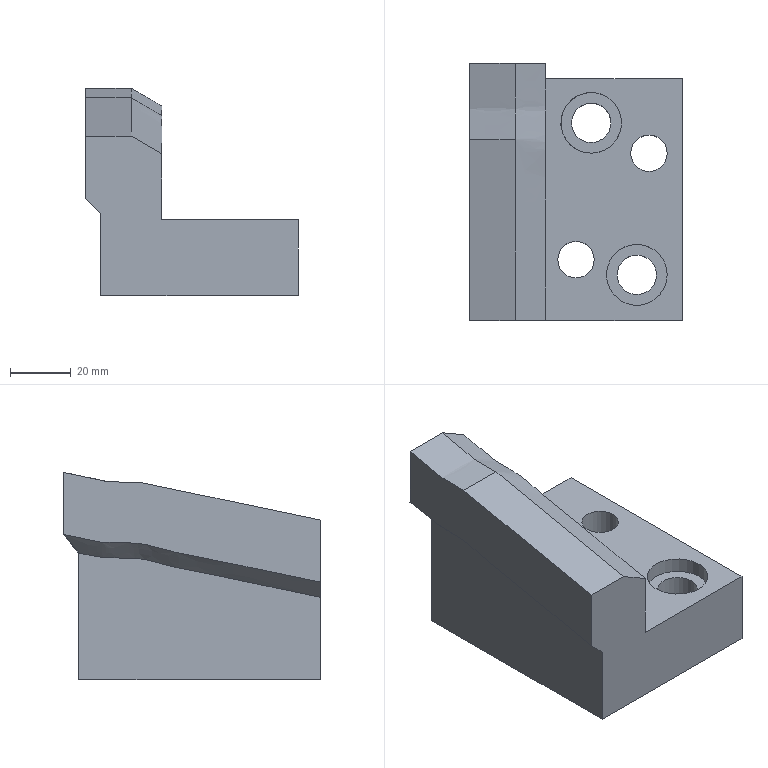Part | NX | features solid 2 | 1 solid | 22 faces | box 70 x 84.485 x 68.169 mm | volume 180874 mm3 | plane 9 | spline 7 | cylinder 6 | commonest cylinder face diameters 12 x2 13 x2 20 x2
STEP:
#1=CARTESIAN_POINT('',(-25.,-719.515,-87.945));
#2=VERTEX_POINT('',#1);
#3=CARTESIAN_POINT('',(-25.,-640.058,-73.347));
#4=VERTEX_POINT('',#3);
#5=CARTESIAN_POINT('',(-25.,-719.515,-87.945));
#6=CARTESIAN_POINT('',(-25.,-712.92,-86.565));
#7=CARTESIAN_POINT('',(-25.,-703.034,-84.459));
#8=CARTESIAN_POINT('',(-25.,-689.828,-81.777));
#9=CARTESIAN_POINT('',(-25.,-679.973,-79.509));
#10=CARTESIAN_POINT('',(-25.,-669.974,-78.004));
#11=CARTESIAN_POINT('',(-25.,-661.914,-75.049));
#12=CARTESIAN_POINT('',(-25.,-655.949,-75.021));
#13=CARTESIAN_POINT('',(-25.,-652.544,-74.98));
#14=CARTESIAN_POINT('',(-25.,-649.12,-75.057));
#15=CARTESIAN_POINT('',(-25.,-644.974,-74.425));
#16=CARTESIAN_POINT('',(-25.,-641.698,-73.697));
#17=CARTESIAN_POINT('',(-25.,-640.058,-73.347));
#18=B_SPLINE_CURVE_WITH_KNOTS('',3,(#5,#6,#7,#8,#9,#10,#11,#12,#13,#14,#15,#16,#17),.UNSPECIFIED.,.F.,.F.,(4,1,1,1,1,1,1,1,1,1,4),(0.2923,0.3125,0.3225,0.3326,0.3427,0.3528,0.3579,0.3604,0.3629,0.368,0.373),.UNSPECIFIED.);
#19=EDGE_CURVE('',#2,#4,#18,.T.);
#20=ORIENTED_EDGE('',*,*,#19,.F.);
#21=CARTESIAN_POINT('',(-30.,-719.515,-82.945));
#22=VERTEX_POINT('',#21);
#23=CARTESIAN_POINT('',(-25.,-719.515,-87.945));
#24=CARTESIAN_POINT('',(-26.667,-719.515,-86.278));
#25=CARTESIAN_POINT('',(-28.333,-719.515,-84.612));
#26=CARTESIAN_POINT('',(-30.,-719.515,-82.945));
#27=B_SPLINE_CURVE_WITH_KNOTS('',3,(#23,#24,#25,#26),.UNSPECIFIED.,.F.,.F.,(4,4),(0.00004375,0.007115),.UNSPECIFIED.);
#28=EDGE_CURVE('',#2,#22,#27,.T.);
#29=ORIENTED_EDGE('',*,*,#28,.T.);
#30=CARTESIAN_POINT('',(-30.,-635.066,-67.29));
#31=VERTEX_POINT('',#30);
#32=CARTESIAN_POINT('',(-30.,-635.066,-67.29));
#33=CARTESIAN_POINT('',(-30.,-636.808,-67.66));
#34=CARTESIAN_POINT('',(-30.,-640.294,-68.391));
#35=CARTESIAN_POINT('',(-30.,-644.645,-69.338));
#36=CARTESIAN_POINT('',(-30.,-648.159,-69.92));
#37=CARTESIAN_POINT('',(-30.,-650.86,-70.019));
#38=CARTESIAN_POINT('',(-30.,-653.581,-69.998));
#39=CARTESIAN_POINT('',(-30.,-657.204,-70.002));
#40=CARTESIAN_POINT('',(-30.,-661.695,-70.263));
#41=CARTESIAN_POINT('',(-30.,-666.893,-71.833));
#42=CARTESIAN_POINT('',(-30.,-672.117,-73.232));
#43=CARTESIAN_POINT('',(-30.,-677.416,-74.141));
#44=CARTESIAN_POINT('',(-30.,-682.694,-75.169));
#45=CARTESIAN_POINT('',(-30.,-687.944,-76.329));
#46=CARTESIAN_POINT('',(-30.,-693.201,-77.456));
#47=CARTESIAN_POINT('',(-30.,-703.735,-79.613));
#48=CARTESIAN_POINT('',(-30.,-712.499,-81.477));
#49=CARTESIAN_POINT('',(-30.,-719.515,-82.945));
#50=B_SPLINE_CURVE_WITH_KNOTS('',3,(#32,#33,#34,#35,#36,#37,#38,#39,#40,#41,#42,#43,#44,#45,#46,#47,#48,#49),.UNSPECIFIED.,.F.,.F.,(4,1,1,1,1,1,1,1,1,1,1,1,1,1,1,4),(0.01003,0.01537,0.02071,0.02338,0.02605,0.02872,0.03139,0.03674,0.04208,0.04742,0.05276,0.0581,0.06344,0.06879,0.07413,0.09549),.UNSPECIFIED.);
#51=EDGE_CURVE('',#31,#22,#50,.T.);
#52=ORIENTED_EDGE('',*,*,#51,.F.);
#53=CARTESIAN_POINT('',(-25.002,-640.058,-73.345));
#54=VERTEX_POINT('',#53);
#55=CARTESIAN_POINT('',(-25.002,-640.058,-73.345));
#56=CARTESIAN_POINT('',(-26.666,-638.393,-71.326));
#57=CARTESIAN_POINT('',(-28.334,-636.73,-69.309));
#58=CARTESIAN_POINT('',(-30.,-635.066,-67.29));
#59=B_SPLINE_CURVE_WITH_KNOTS('',3,(#55,#56,#57,#58),.UNSPECIFIED.,.F.,.F.,(4,4),(0.00005607,0.00936),.UNSPECIFIED.);
#60=EDGE_CURVE('',#54,#31,#59,.T.);
#61=ORIENTED_EDGE('',*,*,#60,.F.);
#62=CARTESIAN_POINT('',(-25.002,-640.058,-73.345));
#63=CARTESIAN_POINT('',(-25.001,-640.058,-73.346));
#64=CARTESIAN_POINT('',(-25.001,-640.058,-73.346));
#65=CARTESIAN_POINT('',(-25.,-640.058,-73.347));
#66=B_SPLINE_CURVE_WITH_KNOTS('',3,(#62,#63,#64,#65),.UNSPECIFIED.,.F.,.F.,(4,4),(0.001559,0.001561),.UNSPECIFIED.);
#67=EDGE_CURVE('',#54,#4,#66,.T.);
#68=ORIENTED_EDGE('',*,*,#67,.T.);
#69=EDGE_LOOP('',(#20,#29,#52,#61,#68));
#70=FACE_BOUND('',#69,.T.);
#71=CARTESIAN_POINT('',(-30.032,-634.561,-67.151));
#72=CARTESIAN_POINT('',(-28.344,-634.561,-68.838));
#73=CARTESIAN_POINT('',(-26.657,-634.561,-70.525));
#74=CARTESIAN_POINT('',(-24.969,-634.561,-72.212));
#75=CARTESIAN_POINT('',(-30.032,-634.924,-67.228));
#76=CARTESIAN_POINT('',(-28.344,-634.925,-68.915));
#77=CARTESIAN_POINT('',(-26.657,-634.925,-70.602));
#78=CARTESIAN_POINT('',(-24.969,-634.925,-72.289));
#79=CARTESIAN_POINT('',(-30.032,-637.021,-67.673));
#80=CARTESIAN_POINT('',(-28.345,-637.021,-69.36));
#81=CARTESIAN_POINT('',(-26.657,-637.021,-71.048));
#82=CARTESIAN_POINT('',(-24.97,-637.021,-72.735));
#83=CARTESIAN_POINT('',(-30.033,-639.862,-68.269));
#84=CARTESIAN_POINT('',(-28.345,-639.862,-69.956));
#85=CARTESIAN_POINT('',(-26.658,-639.862,-71.644));
#86=CARTESIAN_POINT('',(-24.97,-639.862,-73.332));
#87=CARTESIAN_POINT('',(-30.033,-643.326,-69.018));
#88=CARTESIAN_POINT('',(-28.345,-643.326,-70.705));
#89=CARTESIAN_POINT('',(-26.657,-643.326,-72.393));
#90=CARTESIAN_POINT('',(-24.97,-643.326,-74.081));
#91=CARTESIAN_POINT('',(-30.031,-645.56,-69.46));
#92=CARTESIAN_POINT('',(-28.344,-645.56,-71.147));
#93=CARTESIAN_POINT('',(-26.657,-645.56,-72.834));
#94=CARTESIAN_POINT('',(-24.969,-645.56,-74.522));
#95=CARTESIAN_POINT('',(-30.031,-647.563,-69.771));
#96=CARTESIAN_POINT('',(-28.344,-647.563,-71.458));
#97=CARTESIAN_POINT('',(-26.657,-647.563,-73.145));
#98=CARTESIAN_POINT('',(-24.969,-647.563,-74.833));
#99=CARTESIAN_POINT('',(-30.032,-648.821,-69.904));
#100=CARTESIAN_POINT('',(-28.345,-648.821,-71.591));
#101=CARTESIAN_POINT('',(-26.657,-648.821,-73.279));
#102=CARTESIAN_POINT('',(-24.97,-648.821,-74.966));
#103=CARTESIAN_POINT('',(-30.032,-649.831,-69.958));
#104=CARTESIAN_POINT('',(-28.345,-649.831,-71.646));
#105=CARTESIAN_POINT('',(-26.657,-649.831,-73.333));
#106=CARTESIAN_POINT('',(-24.97,-649.831,-75.02));
#107=CARTESIAN_POINT('',(-30.032,-650.716,-69.97));
#108=CARTESIAN_POINT('',(-28.345,-650.716,-71.658));
#109=CARTESIAN_POINT('',(-26.657,-650.716,-73.345));
#110=CARTESIAN_POINT('',(-24.969,-650.716,-75.033));
#111=CARTESIAN_POINT('',(-30.032,-651.476,-69.962));
#112=CARTESIAN_POINT('',(-28.345,-651.476,-71.649));
#113=CARTESIAN_POINT('',(-26.657,-651.476,-73.337));
#114=CARTESIAN_POINT('',(-24.97,-651.476,-75.024));
#115=CARTESIAN_POINT('',(-30.032,-652.488,-69.961));
#116=CARTESIAN_POINT('',(-28.345,-652.488,-71.649));
#117=CARTESIAN_POINT('',(-26.657,-652.488,-73.336));
#118=CARTESIAN_POINT('',(-24.97,-652.488,-75.023));
#119=CARTESIAN_POINT('',(-30.032,-653.627,-69.972));
#120=CARTESIAN_POINT('',(-28.345,-653.627,-71.659));
#121=CARTESIAN_POINT('',(-26.657,-653.627,-73.346));
#122=CARTESIAN_POINT('',(-24.969,-653.627,-75.033));
#123=CARTESIAN_POINT('',(-30.032,-655.146,-69.976));
#124=CARTESIAN_POINT('',(-28.344,-655.146,-71.663));
#125=CARTESIAN_POINT('',(-26.657,-655.146,-73.351));
#126=CARTESIAN_POINT('',(-24.969,-655.146,-75.038));
#127=CARTESIAN_POINT('',(-30.032,-656.665,-69.987));
#128=CARTESIAN_POINT('',(-28.344,-656.665,-71.675));
#129=CARTESIAN_POINT('',(-26.657,-656.665,-73.363));
#130=CARTESIAN_POINT('',(-24.969,-656.665,-75.051));
#131=CARTESIAN_POINT('',(-30.032,-658.185,-70.024));
#132=CARTESIAN_POINT('',(-28.345,-658.185,-71.712));
#133=CARTESIAN_POINT('',(-26.657,-658.185,-73.4));
#134=CARTESIAN_POINT('',(-24.969,-658.185,-75.087));
#135=CARTESIAN_POINT('',(-30.033,-660.707,-70.197));
#136=CARTESIAN_POINT('',(-28.346,-660.707,-71.884));
#137=CARTESIAN_POINT('',(-26.658,-660.707,-73.572));
#138=CARTESIAN_POINT('',(-24.97,-660.707,-75.26));
#139=CARTESIAN_POINT('',(-30.035,-663.428,-70.785));
#140=CARTESIAN_POINT('',(-28.347,-663.428,-72.474));
#141=CARTESIAN_POINT('',(-26.659,-663.428,-74.162));
#142=CARTESIAN_POINT('',(-24.97,-663.428,-75.851));
#143=CARTESIAN_POINT('',(-30.034,-666.726,-71.717));
#144=CARTESIAN_POINT('',(-28.346,-666.726,-73.405));
#145=CARTESIAN_POINT('',(-26.658,-666.726,-75.094));
#146=CARTESIAN_POINT('',(-24.97,-666.726,-76.782));
#147=CARTESIAN_POINT('',(-30.032,-668.669,-72.286));
#148=CARTESIAN_POINT('',(-28.345,-668.669,-73.974));
#149=CARTESIAN_POINT('',(-26.657,-668.669,-75.662));
#150=CARTESIAN_POINT('',(-24.969,-668.669,-77.35));
#151=CARTESIAN_POINT('',(-30.031,-670.876,-72.848));
#152=CARTESIAN_POINT('',(-28.344,-670.876,-74.535));
#153=CARTESIAN_POINT('',(-26.657,-670.876,-76.223));
#154=CARTESIAN_POINT('',(-24.969,-670.876,-77.91));
#155=CARTESIAN_POINT('',(-30.031,-673.966,-73.534));
#156=CARTESIAN_POINT('',(-28.344,-673.966,-75.221));
#157=CARTESIAN_POINT('',(-26.657,-673.966,-76.908));
#158=CARTESIAN_POINT('',(-24.969,-673.966,-78.596));
#159=CARTESIAN_POINT('',(-30.033,-678.959,-74.372));
#160=CARTESIAN_POINT('',(-28.345,-678.959,-76.06));
#161=CARTESIAN_POINT('',(-26.658,-678.959,-77.748));
#162=CARTESIAN_POINT('',(-24.97,-678.959,-79.435));
#163=CARTESIAN_POINT('',(-30.032,-684.905,-75.616));
#164=CARTESIAN_POINT('',(-28.345,-684.905,-77.304));
#165=CARTESIAN_POINT('',(-26.657,-684.904,-78.992));
#166=CARTESIAN_POINT('',(-24.969,-684.904,-80.68));
#167=CARTESIAN_POINT('',(-30.031,-690.834,-76.935));
#168=CARTESIAN_POINT('',(-28.343,-690.834,-78.622));
#169=CARTESIAN_POINT('',(-26.656,-690.834,-80.31));
#170=CARTESIAN_POINT('',(-24.968,-690.834,-81.998));
#171=CARTESIAN_POINT('',(-30.032,-698.768,-78.56));
#172=CARTESIAN_POINT('',(-28.345,-698.768,-80.248));
#173=CARTESIAN_POINT('',(-26.657,-698.768,-81.935));
#174=CARTESIAN_POINT('',(-24.97,-698.768,-83.623));
#175=CARTESIAN_POINT('',(-30.032,-706.694,-80.221));
#176=CARTESIAN_POINT('',(-28.345,-706.694,-81.909));
#177=CARTESIAN_POINT('',(-26.657,-706.694,-83.597));
#178=CARTESIAN_POINT('',(-24.969,-706.694,-85.284));
#179=CARTESIAN_POINT('',(-30.032,-714.438,-81.85));
#180=CARTESIAN_POINT('',(-28.345,-714.438,-83.537));
#181=CARTESIAN_POINT('',(-26.657,-714.438,-85.225));
#182=CARTESIAN_POINT('',(-24.969,-714.438,-86.912));
#183=CARTESIAN_POINT('',(-30.032,-718.22,-82.642));
#184=CARTESIAN_POINT('',(-28.344,-718.22,-84.33));
#185=CARTESIAN_POINT('',(-26.657,-718.22,-86.017));
#186=CARTESIAN_POINT('',(-24.969,-718.22,-87.705));
#187=CARTESIAN_POINT('',(-30.032,-720.021,-83.019));
#188=CARTESIAN_POINT('',(-28.344,-720.021,-84.707));
#189=CARTESIAN_POINT('',(-26.657,-720.021,-86.394));
#190=CARTESIAN_POINT('',(-24.969,-720.021,-88.082));
#191=B_SPLINE_SURFACE_WITH_KNOTS('',3,3,((#71,#72,#73,#74),(#75,#76,#77,#78),(#79,#80,#81,#82),(#83,#84,#85,#86),(#87,#88,#89,#90),(#91,#92,#93,#94),(#95,#96,#97,#98),(#99,#100,#101,#102),(#103,#104,#105,#106),(#107,#108,#109,#110),(#111,#112,#113,#114),(#115,#116,#117,#118),(#119,#120,#121,#122),(#123,#124,#125,#126),(#127,#128,#129,#130),(#131,#132,#133,#134),(#135,#136,#137,#138),(#139,#140,#141,#142),(#143,#144,#145,#146),(#147,#148,#149,#150),(#151,#152,#153,#154),(#155,#156,#157,#158),(#159,#160,#161,#162),(#163,#164,#165,#166),(#167,#168,#169,#170),(#171,#172,#173,#174),(#175,#176,#177,#178),(#179,#180,#181,#182),(#183,#184,#185,#186),(#187,#188,#189,#190)),.RULED_SURF.,.F.,.F.,.F.,(4,1,1,1,1,1,1,1,1,1,1,1,1,1,1,1,1,1,1,1,1,1,1,1,1,1,1,4),(4,4),(0.02447,0.02734,0.04102,0.04688,0.05469,0.05859,0.0625,0.06445,0.06641,0.06934,0.07031,0.07422,0.07812,0.08203,0.08594,0.08984,0.1016,0.1074,0.1162,0.1172,0.125,0.1406,0.1562,0.1719,0.1875,0.2188,0.2344,0.2486),(0.2187,0.7812),.UNSPECIFIED.);
#192=ADVANCED_FACE('',(#70),#191,.F.);
#193=CARTESIAN_POINT('',(-5.,-635.03,-52.606));
#194=VERTEX_POINT('',#193);
#195=CARTESIAN_POINT('',(-5.,-719.515,-68.291));
#196=VERTEX_POINT('',#195);
#197=CARTESIAN_POINT('',(-5.,-635.03,-52.606));
#198=CARTESIAN_POINT('',(-5.,-636.77,-52.978));
#199=CARTESIAN_POINT('',(-5.,-640.248,-53.744));
#200=CARTESIAN_POINT('',(-5.,-644.61,-54.618));
#201=CARTESIAN_POINT('',(-5.,-647.667,-55.216));
#202=CARTESIAN_POINT('',(-5.,-649.392,-55.667));
#203=CARTESIAN_POINT('',(-5.,-650.724,-55.809));
#204=CARTESIAN_POINT('',(-5.,-652.094,-55.746));
#205=CARTESIAN_POINT('',(-5.,-653.904,-55.758));
#206=CARTESIAN_POINT('',(-5.,-656.157,-55.834));
#207=CARTESIAN_POINT('',(-5.,-658.88,-55.798));
#208=CARTESIAN_POINT('',(-5.,-662.476,-55.986));
#209=CARTESIAN_POINT('',(-5.,-666.839,-57.114));
#210=CARTESIAN_POINT('',(-5.,-672.073,-58.475));
#211=CARTESIAN_POINT('',(-5.,-679.122,-59.819));
#212=CARTESIAN_POINT('',(-5.,-687.904,-61.659));
#213=CARTESIAN_POINT('',(-5.,-701.949,-64.628));
#214=CARTESIAN_POINT('',(-5.,-712.49,-66.817));
#215=CARTESIAN_POINT('',(-5.,-719.515,-68.291));
#216=B_SPLINE_CURVE_WITH_KNOTS('',3,(#197,#198,#199,#200,#201,#202,#203,#204,#205,#206,#207,#208,#209,#210,#211,#212,#213,#214,#215),.UNSPECIFIED.,.F.,.F.,(4,1,1,1,1,1,1,1,1,1,1,1,1,1,1,1,4),(0.009985,0.01532,0.02066,0.02333,0.02467,0.026,0.02734,0.02867,0.03134,0.03401,0.03668,0.04202,0.04736,0.0527,0.06337,0.07405,0.09541),.UNSPECIFIED.);
#217=EDGE_CURVE('',#194,#196,#216,.T.);
#218=ORIENTED_EDGE('',*,*,#217,.T.);
#219=CARTESIAN_POINT('',(-5.,-719.515,-90.));
#220=VERTEX_POINT('',#219);
#221=CARTESIAN_POINT('',(-5.,-719.515,-202.54));
#222=DIRECTION('',(0.,0.,-1.));
#223=VECTOR('',#222,1000.);
#224=LINE('',#221,#223);
#225=EDGE_CURVE('',#196,#220,#224,.T.);
#226=ORIENTED_EDGE('',*,*,#225,.T.);
#227=CARTESIAN_POINT('',(-5.,-640.03,-90.));
#228=VERTEX_POINT('',#227);
#229=CARTESIAN_POINT('',(-5.,-625.255,-90.));
#230=DIRECTION('',(0.,1.,0.));
#231=VECTOR('',#230,1000.);
#232=LINE('',#229,#231);
#233=EDGE_CURVE('',#220,#228,#232,.T.);
#234=ORIENTED_EDGE('',*,*,#233,.T.);
#235=CARTESIAN_POINT('',(-5.,-640.03,-73.416));
#236=VERTEX_POINT('',#235);
#237=CARTESIAN_POINT('',(-5.,-640.03,-161.122));
#238=DIRECTION('',(0.,0.,1.));
#239=VECTOR('',#238,1000.);
#240=LINE('',#237,#239);
#241=EDGE_CURVE('',#228,#236,#240,.T.);
#242=ORIENTED_EDGE('',*,*,#241,.T.);
#243=CARTESIAN_POINT('',(-5.,-635.03,-67.38));
#244=VERTEX_POINT('',#243);
#245=CARTESIAN_POINT('',(-5.,-635.03,-67.38));
#246=CARTESIAN_POINT('',(-5.,-636.696,-69.392));
#247=CARTESIAN_POINT('',(-5.,-638.363,-71.404));
#248=CARTESIAN_POINT('',(-5.,-640.03,-73.416));
#249=B_SPLINE_CURVE_WITH_KNOTS('',3,(#245,#246,#247,#248),.UNSPECIFIED.,.F.,.F.,(4,4),(0.00004752,0.007885),.UNSPECIFIED.);
#250=EDGE_CURVE('',#244,#236,#249,.T.);
#251=ORIENTED_EDGE('',*,*,#250,.F.);
#252=CARTESIAN_POINT('',(-5.,-635.03,-32.126));
#253=DIRECTION('',(0.,0.,-1.));
#254=VECTOR('',#253,1000.);
#255=LINE('',#252,#254);
#256=EDGE_CURVE('',#194,#244,#255,.T.);
#257=ORIENTED_EDGE('',*,*,#256,.F.);
#258=EDGE_LOOP('',(#218,#226,#234,#242,#251,#257));
#259=FACE_BOUND('',#258,.T.);
#260=CARTESIAN_POINT('',(-5.,-625.255,-202.54));
#261=DIRECTION('',(-1.,0.,0.));
#262=DIRECTION('',(0.,-1.,0.));
#263=AXIS2_PLACEMENT_3D('',#260,#261,#262);
#264=PLANE('',#263);
#265=ADVANCED_FACE('',(#259),#264,.F.);
#266=CARTESIAN_POINT('',(-15.,-719.515,-62.518));
#267=VERTEX_POINT('',#266);
#268=CARTESIAN_POINT('',(-5.,-719.515,-68.291));
#269=CARTESIAN_POINT('',(-8.333,-719.515,-66.367));
#270=CARTESIAN_POINT('',(-11.667,-719.515,-64.442));
#271=CARTESIAN_POINT('',(-15.,-719.515,-62.518));
#272=B_SPLINE_CURVE_WITH_KNOTS('',3,(#268,#269,#270,#271),.UNSPECIFIED.,.F.,.F.,(4,4),(0.00007099,0.01162),.UNSPECIFIED.);
#273=EDGE_CURVE('',#196,#267,#272,.T.);
#274=ORIENTED_EDGE('',*,*,#273,.F.);
#275=ORIENTED_EDGE('',*,*,#217,.F.);
#276=CARTESIAN_POINT('',(-15.,-635.043,-46.832));
#277=VERTEX_POINT('',#276);
#278=CARTESIAN_POINT('',(-5.,-635.03,-52.606));
#279=CARTESIAN_POINT('',(-8.333,-635.034,-50.681));
#280=CARTESIAN_POINT('',(-11.667,-635.038,-48.756));
#281=CARTESIAN_POINT('',(-15.,-635.043,-46.831));
#282=B_SPLINE_CURVE_WITH_KNOTS('',3,(#278,#279,#280,#281),.UNSPECIFIED.,.F.,.F.,(4,4),(0.00009309,0.01164),.UNSPECIFIED.);
#283=EDGE_CURVE('',#194,#277,#282,.T.);
#284=ORIENTED_EDGE('',*,*,#283,.T.);
#285=CARTESIAN_POINT('',(-15.,-660.065,-50.074));
#286=VERTEX_POINT('',#285);
#287=CARTESIAN_POINT('',(-15.,-635.043,-46.831));
#288=CARTESIAN_POINT('',(-15.,-637.11,-47.266));
#289=CARTESIAN_POINT('',(-15.,-640.211,-47.917));
#290=CARTESIAN_POINT('',(-15.,-644.341,-48.813));
#291=CARTESIAN_POINT('',(-15.,-646.939,-49.284));
#292=CARTESIAN_POINT('',(-15.,-648.991,-49.795));
#293=CARTESIAN_POINT('',(-15.,-650.556,-50.052));
#294=CARTESIAN_POINT('',(-15.001,-652.145,-49.971));
#295=CARTESIAN_POINT('',(-15.,-654.256,-50.03));
#296=CARTESIAN_POINT('',(-15.,-656.37,-50.017));
#297=CARTESIAN_POINT('',(-15.,-658.479,-50.079));
#298=CARTESIAN_POINT('',(-15.,-659.542,-50.012));
#299=CARTESIAN_POINT('',(-15.,-660.064,-50.078));
#300=B_SPLINE_CURVE_WITH_KNOTS('',3,(#287,#288,#289,#290,#291,#292,#293,#294,#295,#296,#297,#298,#299),.UNSPECIFIED.,.F.,.F.,(4,1,1,1,1,1,1,1,1,1,4),(0.,0.25,0.375,0.5,0.5625,0.625,0.6875,0.75,0.875,0.9375,1.),.UNSPECIFIED.);
#301=EDGE_CURVE('',#286,#277,#300,.F.);
#302=ORIENTED_EDGE('',*,*,#301,.F.);
#303=CARTESIAN_POINT('',(-15.,-660.064,-50.078));
#304=CARTESIAN_POINT('',(-15.,-660.69,-50.156));
#305=CARTESIAN_POINT('',(-15.,-661.921,-50.476));
#306=CARTESIAN_POINT('',(-15.,-664.398,-50.975));
#307=CARTESIAN_POINT('',(-15.,-667.489,-51.629));
#308=CARTESIAN_POINT('',(-15.,-671.203,-52.399));
#309=CARTESIAN_POINT('',(-15.,-676.157,-53.436));
#310=CARTESIAN_POINT('',(-15.,-682.352,-54.736));
#311=CARTESIAN_POINT('',(-15.,-692.263,-56.815));
#312=CARTESIAN_POINT('',(-15.,-704.65,-59.406));
#313=CARTESIAN_POINT('',(-15.,-714.56,-61.481));
#314=CARTESIAN_POINT('',(-15.,-719.515,-62.518));
#315=B_SPLINE_CURVE_WITH_KNOTS('',3,(#303,#304,#305,#306,#307,#308,#309,#310,#311,#312,#313,#314),.UNSPECIFIED.,.F.,.F.,(4,1,1,1,1,1,1,1,1,4),(0.,0.005548,0.0111,0.02219,0.03329,0.04438,0.06657,0.08876,0.1331,0.1775),.UNSPECIFIED.);
#316=EDGE_CURVE('',#286,#267,#315,.T.);
#317=ORIENTED_EDGE('',*,*,#316,.T.);
#318=EDGE_LOOP('',(#274,#275,#284,#302,#317));
#319=FACE_BOUND('',#318,.T.);
#320=CARTESIAN_POINT('',(-15.,-634.525,-46.722));
#321=CARTESIAN_POINT('',(-11.646,-634.525,-48.659));
#322=CARTESIAN_POINT('',(-8.293,-634.524,-50.596));
#323=CARTESIAN_POINT('',(-4.939,-634.524,-52.533));
#324=CARTESIAN_POINT('',(-15.,-634.903,-46.802));
#325=CARTESIAN_POINT('',(-11.646,-634.903,-48.739));
#326=CARTESIAN_POINT('',(-8.293,-634.903,-50.677));
#327=CARTESIAN_POINT('',(-4.939,-634.903,-52.614));
#328=CARTESIAN_POINT('',(-15.,-637.016,-47.246));
#329=CARTESIAN_POINT('',(-11.646,-637.015,-49.187));
#330=CARTESIAN_POINT('',(-8.291,-637.015,-51.127));
#331=CARTESIAN_POINT('',(-4.936,-637.014,-53.067));
#332=CARTESIAN_POINT('',(-15.,-639.871,-47.852));
#333=CARTESIAN_POINT('',(-11.645,-639.869,-49.799));
#334=CARTESIAN_POINT('',(-8.289,-639.867,-51.747));
#335=CARTESIAN_POINT('',(-4.933,-639.865,-53.694));
#336=CARTESIAN_POINT('',(-15.,-643.337,-48.587));
#337=CARTESIAN_POINT('',(-11.645,-643.337,-50.526));
#338=CARTESIAN_POINT('',(-8.29,-643.337,-52.464));
#339=CARTESIAN_POINT('',(-4.935,-643.336,-54.402));
#340=CARTESIAN_POINT('',(-15.,-645.444,-49.024));
#341=CARTESIAN_POINT('',(-11.646,-645.445,-50.954));
#342=CARTESIAN_POINT('',(-8.293,-645.446,-52.885));
#343=CARTESIAN_POINT('',(-4.939,-645.447,-54.816));
#344=CARTESIAN_POINT('',(-15.,-646.934,-49.318));
#345=CARTESIAN_POINT('',(-11.647,-646.935,-51.248));
#346=CARTESIAN_POINT('',(-8.293,-646.936,-53.178));
#347=CARTESIAN_POINT('',(-4.94,-646.938,-55.108));
#348=CARTESIAN_POINT('',(-15.,-647.678,-49.469));
#349=CARTESIAN_POINT('',(-11.646,-647.678,-51.404));
#350=CARTESIAN_POINT('',(-8.293,-647.679,-53.339));
#351=CARTESIAN_POINT('',(-4.939,-647.679,-55.273));
#352=CARTESIAN_POINT('',(-15.,-648.296,-49.603));
#353=CARTESIAN_POINT('',(-11.646,-648.296,-51.542));
#354=CARTESIAN_POINT('',(-8.292,-648.295,-53.481));
#355=CARTESIAN_POINT('',(-4.938,-648.294,-55.42));
#356=CARTESIAN_POINT('',(-15.,-648.911,-49.757));
#357=CARTESIAN_POINT('',(-11.646,-648.91,-51.696));
#358=CARTESIAN_POINT('',(-8.292,-648.91,-53.634));
#359=CARTESIAN_POINT('',(-4.938,-648.91,-55.572));
#360=CARTESIAN_POINT('',(-15.,-649.653,-49.919));
#361=CARTESIAN_POINT('',(-11.646,-649.653,-51.854));
#362=CARTESIAN_POINT('',(-8.292,-649.653,-53.79));
#363=CARTESIAN_POINT('',(-4.938,-649.653,-55.725));
#364=CARTESIAN_POINT('',(-15.,-650.408,-50.02));
#365=CARTESIAN_POINT('',(-11.646,-650.408,-51.952));
#366=CARTESIAN_POINT('',(-8.292,-650.408,-53.885));
#367=CARTESIAN_POINT('',(-4.939,-650.408,-55.818));
#368=CARTESIAN_POINT('',(-15.,-651.294,-49.976));
#369=CARTESIAN_POINT('',(-11.646,-651.294,-51.921));
#370=CARTESIAN_POINT('',(-8.293,-651.294,-53.866));
#371=CARTESIAN_POINT('',(-4.939,-651.294,-55.811));
#372=CARTESIAN_POINT('',(-15.,-652.053,-49.991));
#373=CARTESIAN_POINT('',(-11.646,-652.054,-51.925));
#374=CARTESIAN_POINT('',(-8.293,-652.054,-53.858));
#375=CARTESIAN_POINT('',(-4.939,-652.054,-55.792));
#376=CARTESIAN_POINT('',(-15.001,-652.813,-50.001));
#377=CARTESIAN_POINT('',(-11.646,-652.813,-51.93));
#378=CARTESIAN_POINT('',(-8.292,-652.813,-53.859));
#379=CARTESIAN_POINT('',(-4.938,-652.813,-55.788));
#380=CARTESIAN_POINT('',(-15.,-653.825,-50.01));
#381=CARTESIAN_POINT('',(-11.646,-653.825,-51.939));
#382=CARTESIAN_POINT('',(-8.292,-653.826,-53.869));
#383=CARTESIAN_POINT('',(-4.938,-653.826,-55.798));
#384=CARTESIAN_POINT('',(-15.,-654.964,-50.018));
#385=CARTESIAN_POINT('',(-11.646,-654.964,-51.953));
#386=CARTESIAN_POINT('',(-8.292,-654.964,-53.889));
#387=CARTESIAN_POINT('',(-4.939,-654.964,-55.824));
#388=CARTESIAN_POINT('',(-15.,-656.23,-50.029));
#389=CARTESIAN_POINT('',(-11.646,-656.23,-51.97));
#390=CARTESIAN_POINT('',(-8.292,-656.23,-53.911));
#391=CARTESIAN_POINT('',(-4.939,-656.23,-55.852));
#392=CARTESIAN_POINT('',(-15.,-657.495,-50.048));
#393=CARTESIAN_POINT('',(-11.646,-657.495,-51.987));
#394=CARTESIAN_POINT('',(-8.292,-657.495,-53.925));
#395=CARTESIAN_POINT('',(-4.939,-657.495,-55.864));
#396=CARTESIAN_POINT('',(-15.,-658.555,-50.058));
#397=CARTESIAN_POINT('',(-11.646,-658.555,-51.993));
#398=CARTESIAN_POINT('',(-8.292,-658.555,-53.929));
#399=CARTESIAN_POINT('',(-4.939,-658.555,-55.864));
#400=CARTESIAN_POINT('',(-15.,-659.315,-50.051));
#401=CARTESIAN_POINT('',(-11.646,-659.315,-51.988));
#402=CARTESIAN_POINT('',(-8.292,-659.315,-53.925));
#403=CARTESIAN_POINT('',(-4.939,-659.315,-55.862));
#404=CARTESIAN_POINT('',(-15.,-659.663,-50.05));
#405=CARTESIAN_POINT('',(-11.646,-659.663,-51.989));
#406=CARTESIAN_POINT('',(-8.292,-659.663,-53.928));
#407=CARTESIAN_POINT('',(-4.939,-659.663,-55.866));
#408=CARTESIAN_POINT('',(-15.,-659.924,-50.06));
#409=CARTESIAN_POINT('',(-11.646,-659.924,-51.998));
#410=CARTESIAN_POINT('',(-8.292,-659.924,-53.936));
#411=CARTESIAN_POINT('',(-4.939,-659.924,-55.874));
#412=CARTESIAN_POINT('',(-15.,-660.19,-50.092));
#413=CARTESIAN_POINT('',(-11.646,-660.191,-52.024));
#414=CARTESIAN_POINT('',(-8.292,-660.191,-53.956));
#415=CARTESIAN_POINT('',(-4.939,-660.192,-55.889));
#416=CARTESIAN_POINT('',(-15.,-660.53,-50.172));
#417=CARTESIAN_POINT('',(-11.646,-660.533,-52.087));
#418=CARTESIAN_POINT('',(-8.293,-660.536,-54.002));
#419=CARTESIAN_POINT('',(-4.939,-660.538,-55.918));
#420=CARTESIAN_POINT('',(-15.,-661.467,-50.359));
#421=CARTESIAN_POINT('',(-11.646,-661.475,-52.242));
#422=CARTESIAN_POINT('',(-8.293,-661.483,-54.125));
#423=CARTESIAN_POINT('',(-4.939,-661.49,-56.008));
#424=CARTESIAN_POINT('',(-15.,-662.689,-50.622));
#425=CARTESIAN_POINT('',(-11.647,-662.701,-52.481));
#426=CARTESIAN_POINT('',(-8.293,-662.712,-54.34));
#427=CARTESIAN_POINT('',(-4.94,-662.724,-56.199));
#428=CARTESIAN_POINT('',(-15.,-664.73,-51.053));
#429=CARTESIAN_POINT('',(-11.647,-664.743,-52.908));
#430=CARTESIAN_POINT('',(-8.294,-664.757,-54.763));
#431=CARTESIAN_POINT('',(-4.941,-664.77,-56.619));
#432=CARTESIAN_POINT('',(-15.,-667.08,-51.541));
#433=CARTESIAN_POINT('',(-11.647,-667.089,-53.432));
#434=CARTESIAN_POINT('',(-8.293,-667.099,-55.324));
#435=CARTESIAN_POINT('',(-4.94,-667.108,-57.215));
#436=CARTESIAN_POINT('',(-15.,-669.556,-52.056));
#437=CARTESIAN_POINT('',(-11.646,-669.557,-53.989));
#438=CARTESIAN_POINT('',(-8.292,-669.557,-55.922));
#439=CARTESIAN_POINT('',(-4.939,-669.558,-57.856));
#440=CARTESIAN_POINT('',(-15.,-672.527,-52.676));
#441=CARTESIAN_POINT('',(-11.646,-672.521,-54.641));
#442=CARTESIAN_POINT('',(-8.292,-672.516,-56.605));
#443=CARTESIAN_POINT('',(-4.938,-672.51,-58.569));
#444=CARTESIAN_POINT('',(-15.,-675.499,-53.299));
#445=CARTESIAN_POINT('',(-11.646,-675.496,-55.254));
#446=CARTESIAN_POINT('',(-8.292,-675.493,-57.21));
#447=CARTESIAN_POINT('',(-4.938,-675.49,-59.165));
#448=CARTESIAN_POINT('',(-15.,-678.472,-53.922));
#449=CARTESIAN_POINT('',(-11.646,-678.472,-55.864));
#450=CARTESIAN_POINT('',(-8.292,-678.471,-57.805));
#451=CARTESIAN_POINT('',(-4.939,-678.471,-59.747));
#452=CARTESIAN_POINT('',(-15.,-681.446,-54.546));
#453=CARTESIAN_POINT('',(-11.646,-681.447,-56.477));
#454=CARTESIAN_POINT('',(-8.293,-681.448,-58.409));
#455=CARTESIAN_POINT('',(-4.939,-681.449,-60.34));
#456=CARTESIAN_POINT('',(-15.,-685.41,-55.378));
#457=CARTESIAN_POINT('',(-11.646,-685.411,-57.309));
#458=CARTESIAN_POINT('',(-8.293,-685.412,-59.24));
#459=CARTESIAN_POINT('',(-4.939,-685.413,-61.171));
#460=CARTESIAN_POINT('',(-15.,-690.861,-56.521));
#461=CARTESIAN_POINT('',(-11.646,-690.861,-58.454));
#462=CARTESIAN_POINT('',(-8.292,-690.862,-60.388));
#463=CARTESIAN_POINT('',(-4.939,-690.862,-62.322));
#464=CARTESIAN_POINT('',(-15.,-698.789,-58.18));
#465=CARTESIAN_POINT('',(-11.646,-698.789,-60.118));
#466=CARTESIAN_POINT('',(-8.293,-698.788,-62.056));
#467=CARTESIAN_POINT('',(-4.939,-698.787,-63.994));
#468=CARTESIAN_POINT('',(-15.,-708.509,-60.213));
#469=CARTESIAN_POINT('',(-11.646,-708.509,-62.148));
#470=CARTESIAN_POINT('',(-8.291,-708.509,-64.083));
#471=CARTESIAN_POINT('',(-4.937,-708.51,-66.018));
#472=CARTESIAN_POINT('',(-15.,-716.247,-61.834));
#473=CARTESIAN_POINT('',(-11.646,-716.247,-63.769));
#474=CARTESIAN_POINT('',(-8.292,-716.247,-65.705));
#475=CARTESIAN_POINT('',(-4.939,-716.247,-67.641));
#476=CARTESIAN_POINT('',(-15.,-720.021,-62.624));
#477=CARTESIAN_POINT('',(-11.646,-720.021,-64.56));
#478=CARTESIAN_POINT('',(-8.293,-720.021,-66.496));
#479=CARTESIAN_POINT('',(-4.939,-720.021,-68.433));
#480=B_SPLINE_SURFACE_WITH_KNOTS('',3,3,((#320,#321,#322,#323),(#324,#325,#326,#327),(#328,#329,#330,#331),(#332,#333,#334,#335),(#336,#337,#338,#339),(#340,#341,#342,#343),(#344,#345,#346,#347),(#348,#349,#350,#351),(#352,#353,#354,#355),(#356,#357,#358,#359),(#360,#361,#362,#363),(#364,#365,#366,#367),(#368,#369,#370,#371),(#372,#373,#374,#375),(#376,#377,#378,#379),(#380,#381,#382,#383),(#384,#385,#386,#387),(#388,#389,#390,#391),(#392,#393,#394,#395),(#396,#397,#398,#399),(#400,#401,#402,#403),(#404,#405,#406,#407),(#408,#409,#410,#411),(#412,#413,#414,#415),(#416,#417,#418,#419),(#420,#421,#422,#423),(#424,#425,#426,#427),(#428,#429,#430,#431),(#432,#433,#434,#435),(#436,#437,#438,#439),(#440,#441,#442,#443),(#444,#445,#446,#447),(#448,#449,#450,#451),(#452,#453,#454,#455),(#456,#457,#458,#459),(#460,#461,#462,#463),(#464,#465,#466,#467),(#468,#469,#470,#471),(#472,#473,#474,#475),(#476,#477,#478,#479)),.RULED_SURF.,.F.,.F.,.F.,(4,1,1,1,1,1,1,1,1,1,1,1,1,1,1,1,1,1,1,1,1,1,1,1,1,1,1,1,1,1,1,1,1,1,1,1,1,4),(4,4),(0.02436,0.02734,0.04102,0.04688,0.05469,0.05762,0.05859,0.06055,0.0625,0.06348,0.06641,0.06836,0.07031,0.07227,0.07422,0.07812,0.08105,0.08398,0.08789,0.08923,0.08984,0.09058,0.09125,0.09192,0.09326,0.09863,0.1016,0.1094,0.1172,0.1211,0.1328,0.1406,0.1445,0.1562,0.1719,0.1875,0.2188,0.2485),(0.,0.8384),.UNSPECIFIED.);
#481=ADVANCED_FACE('',(#319),#480,.T.);
#482=ORIENTED_EDGE('',*,*,#51,.T.);
#483=CARTESIAN_POINT('',(-30.,-719.515,-62.518));
#484=VERTEX_POINT('',#483);
#485=CARTESIAN_POINT('',(-30.,-719.515,-42.243));
#486=DIRECTION('',(0.,0.,1.));
#487=VECTOR('',#486,1000.);
#488=LINE('',#485,#487);
#489=EDGE_CURVE('',#22,#484,#488,.T.);
#490=ORIENTED_EDGE('',*,*,#489,.T.);
#491=CARTESIAN_POINT('',(-30.,-660.065,-50.071));
#492=VERTEX_POINT('',#491);
#493=CARTESIAN_POINT('',(-30.,-625.147,-42.76));
#494=DIRECTION('',(0.,-0.9788,-0.2049));
#495=VECTOR('',#494,1000.);
#496=LINE('',#493,#495);
#497=EDGE_CURVE('',#492,#484,#496,.T.);
#498=ORIENTED_EDGE('',*,*,#497,.F.);
#499=CARTESIAN_POINT('',(-30.,-635.065,-46.837));
#500=VERTEX_POINT('',#499);
#501=CARTESIAN_POINT('',(-30.,-660.065,-50.071));
#502=CARTESIAN_POINT('',(-30.,-659.942,-50.065));
#503=CARTESIAN_POINT('',(-30.,-659.675,-50.055));
#504=CARTESIAN_POINT('',(-30.,-659.315,-50.054));
#505=CARTESIAN_POINT('',(-30.,-659.12,-50.055));
#506=CARTESIAN_POINT('',(-30.,-658.883,-50.056));
#507=CARTESIAN_POINT('',(-30.,-658.619,-50.059));
#508=CARTESIAN_POINT('',(-30.,-658.445,-50.06));
#509=CARTESIAN_POINT('',(-30.,-658.134,-50.06));
#510=CARTESIAN_POINT('',(-30.,-657.65,-50.054));
#511=CARTESIAN_POINT('',(-30.,-657.453,-50.051));
#512=CARTESIAN_POINT('',(-30.,-656.941,-50.042));
#513=CARTESIAN_POINT('',(-30.,-656.935,-50.042));
#514=CARTESIAN_POINT('',(-30.,-656.716,-50.039));
#515=CARTESIAN_POINT('',(-30.,-656.488,-50.036));
#516=CARTESIAN_POINT('',(-30.,-656.158,-50.031));
#517=CARTESIAN_POINT('',(-30.,-655.766,-50.027));
#518=CARTESIAN_POINT('',(-30.,-655.279,-50.023));
#519=CARTESIAN_POINT('',(-30.,-655.019,-50.02));
#520=CARTESIAN_POINT('',(-30.,-654.507,-50.017));
#521=CARTESIAN_POINT('',(-30.,-653.919,-50.013));
#522=CARTESIAN_POINT('',(-30.,-653.217,-50.008));
#523=CARTESIAN_POINT('',(-30.,-652.984,-50.006));
#524=CARTESIAN_POINT('',(-30.,-652.501,-50.001));
#525=CARTESIAN_POINT('',(-30.,-652.046,-49.994));
#526=CARTESIAN_POINT('',(-30.,-651.352,-49.979));
#527=CARTESIAN_POINT('',(-30.,-650.564,-50.012));
#528=CARTESIAN_POINT('',(-30.,-649.927,-49.976));
#529=CARTESIAN_POINT('',(-30.,-649.43,-49.868));
#530=CARTESIAN_POINT('',(-30.,-649.27,-49.829));
#531=CARTESIAN_POINT('',(-30.,-649.037,-49.772));
#532=CARTESIAN_POINT('',(-30.,-649.012,-49.766));
#533=CARTESIAN_POINT('',(-30.,-648.823,-49.72));
#534=CARTESIAN_POINT('',(-30.,-648.596,-49.668));
#535=CARTESIAN_POINT('',(-30.,-648.278,-49.599));
#536=CARTESIAN_POINT('',(-30.,-648.071,-49.556));
#537=CARTESIAN_POINT('',(-30.,-647.818,-49.504));
#538=CARTESIAN_POINT('',(-30.,-647.746,-49.49));
#539=CARTESIAN_POINT('',(-30.,-647.338,-49.407));
#540=CARTESIAN_POINT('',(-30.,-647.133,-49.365));
#541=CARTESIAN_POINT('',(-30.,-646.618,-49.26));
#542=CARTESIAN_POINT('',(-30.,-646.003,-49.134));
#543=CARTESIAN_POINT('',(-30.,-645.216,-48.972));
#544=CARTESIAN_POINT('',(-30.,-644.323,-48.786));
#545=CARTESIAN_POINT('',(-30.,-643.763,-48.668));
#546=CARTESIAN_POINT('',(-30.,-643.242,-48.559));
#547=CARTESIAN_POINT('',(-30.,-642.772,-48.46));
#548=CARTESIAN_POINT('',(-30.,-642.533,-48.41));
#549=CARTESIAN_POINT('',(-30.,-642.037,-48.305));
#550=CARTESIAN_POINT('',(-30.,-641.298,-48.149));
#551=CARTESIAN_POINT('',(-30.,-640.192,-47.916));
#552=CARTESIAN_POINT('',(-30.,-639.352,-47.739));
#553=CARTESIAN_POINT('',(-30.,-638.784,-47.619));
#554=CARTESIAN_POINT('',(-30.,-638.381,-47.534));
#555=CARTESIAN_POINT('',(-30.,-638.221,-47.5));
#556=CARTESIAN_POINT('',(-30.,-637.718,-47.394));
#557=CARTESIAN_POINT('',(-30.,-637.187,-47.282));
#558=CARTESIAN_POINT('',(-30.,-636.241,-47.084));
#559=CARTESIAN_POINT('',(-30.,-635.52,-46.932));
#560=CARTESIAN_POINT('',(-30.,-635.065,-46.837));
#561=B_SPLINE_CURVE_WITH_KNOTS('',3,(#501,#502,#503,#504,#505,#506,#507,#508,#509,#510,#511,#512,#513,#514,#515,#516,#517,#518,#519,#520,#521,#522,#523,#524,#525,#526,#527,#528,#529,#530,#531,#532,#533,#534,#535,#536,#537,#538,#539,#540,#541,#542,#543,#544,#545,#546,#547,#548,#549,#550,#551,#552,#553,#554,#555,#556,#557,#558,#559,#560),.UNSPECIFIED.,.F.,.F.,(4,1,1,1,1,1,1,1,1,1,1,1,1,1,1,1,1,1,1,1,1,1,1,1,1,1,1,1,1,1,1,1,1,1,1,1,1,1,1,1,1,1,1,1,1,1,1,1,1,1,1,1,1,1,1,1,1,4),(0.,0.01562,0.03125,0.03906,0.04688,0.05469,0.0625,0.07812,0.09375,0.1094,0.1172,0.125,0.1328,0.1406,0.1562,0.1719,0.1875,0.2031,0.2188,0.25,0.2656,0.2812,0.2969,0.3125,0.3438,0.375,0.4062,0.4219,0.4297,0.4336,0.4375,0.4453,0.4531,0.4688,0.4766,0.4844,0.4922,0.5,0.5156,0.5312,0.5625,0.5938,0.625,0.6562,0.6719,0.6875,0.7031,0.7188,0.75,0.7812,0.8125,0.8438,0.8594,0.875,0.8906,0.9062,0.9375,1.),.UNSPECIFIED.);
#562=EDGE_CURVE('',#492,#500,#561,.T.);
#563=ORIENTED_EDGE('',*,*,#562,.T.);
#564=CARTESIAN_POINT('',(-30.,-635.065,-67.289));
#565=VERTEX_POINT('',#564);
#566=CARTESIAN_POINT('',(-30.,-635.065,-32.126));
#567=DIRECTION('',(0.,0.,-1.));
#568=VECTOR('',#567,1000.);
#569=LINE('',#566,#568);
#570=EDGE_CURVE('',#565,#500,#569,.F.);
#571=ORIENTED_EDGE('',*,*,#570,.F.);
#572=CARTESIAN_POINT('',(-30.,-635.066,-67.29));
#573=CARTESIAN_POINT('',(-30.,-635.066,-67.29));
#574=CARTESIAN_POINT('',(-30.,-635.065,-67.29));
#575=CARTESIAN_POINT('',(-30.,-635.065,-67.289));
#576=B_SPLINE_CURVE_WITH_KNOTS('',3,(#572,#573,#574,#575),.UNSPECIFIED.,.F.,.F.,(4,4),(0.007884,0.007885),.UNSPECIFIED.);
#577=EDGE_CURVE('',#31,#565,#576,.T.);
#578=ORIENTED_EDGE('',*,*,#577,.F.);
#579=EDGE_LOOP('',(#482,#490,#498,#563,#571,#578));
#580=FACE_BOUND('',#579,.T.);
#581=CARTESIAN_POINT('',(-30.,-625.255,-42.243));
#582=DIRECTION('',(1.,0.,0.));
#583=DIRECTION('',(0.,1.,0.));
#584=AXIS2_PLACEMENT_3D('',#581,#582,#583);
#585=PLANE('',#584);
#586=ADVANCED_FACE('',(#580),#585,.F.);
#587=ORIENTED_EDGE('',*,*,#562,.F.);
#588=CARTESIAN_POINT('',(81.239,-660.065,-50.071));
#589=DIRECTION('',(1.,0.,-0.000000007));
#590=VECTOR('',#589,1000.);
#591=LINE('',#588,#590);
#592=EDGE_CURVE('',#492,#286,#591,.T.);
#593=ORIENTED_EDGE('',*,*,#592,.T.);
#594=ORIENTED_EDGE('',*,*,#301,.T.);
#595=CARTESIAN_POINT('',(-15.,-635.043,-46.832));
#596=CARTESIAN_POINT('',(-20.,-635.05,-46.834));
#597=CARTESIAN_POINT('',(-25.,-635.057,-46.835));
#598=CARTESIAN_POINT('',(-30.,-635.065,-46.837));
#599=B_SPLINE_CURVE_WITH_KNOTS('',3,(#595,#596,#597,#598),.UNSPECIFIED.,.F.,.F.,(4,4),(0.,1.),.UNSPECIFIED.);
#600=EDGE_CURVE('',#277,#500,#599,.T.);
#601=ORIENTED_EDGE('',*,*,#600,.T.);
#602=EDGE_LOOP('',(#587,#593,#594,#601));
#603=FACE_BOUND('',#602,.T.);
#604=CARTESIAN_POINT('',(-30.,-635.065,-46.837));
#605=CARTESIAN_POINT('',(-25.,-635.058,-46.835));
#606=CARTESIAN_POINT('',(-20.,-635.05,-46.834));
#607=CARTESIAN_POINT('',(-15.,-635.043,-46.832));
#608=CARTESIAN_POINT('',(-30.,-637.131,-47.27));
#609=CARTESIAN_POINT('',(-25.,-637.124,-47.268));
#610=CARTESIAN_POINT('',(-20.,-637.117,-47.267));
#611=CARTESIAN_POINT('',(-15.,-637.111,-47.265));
#612=CARTESIAN_POINT('',(-30.,-641.261,-48.142));
#613=CARTESIAN_POINT('',(-25.,-641.256,-48.14));
#614=CARTESIAN_POINT('',(-20.,-641.25,-48.139));
#615=CARTESIAN_POINT('',(-15.,-641.245,-48.137));
#616=CARTESIAN_POINT('',(-30.,-645.908,-49.122));
#617=CARTESIAN_POINT('',(-25.,-645.904,-49.121));
#618=CARTESIAN_POINT('',(-20.,-645.9,-49.119));
#619=CARTESIAN_POINT('',(-15.,-645.896,-49.118));
#620=CARTESIAN_POINT('',(-30.,-648.753,-49.692));
#621=CARTESIAN_POINT('',(-25.,-648.75,-49.691));
#622=CARTESIAN_POINT('',(-20.,-648.746,-49.691));
#623=CARTESIAN_POINT('',(-15.,-648.743,-49.69));
#624=CARTESIAN_POINT('',(-30.,-649.776,-49.962));
#625=CARTESIAN_POINT('',(-25.,-649.773,-49.962));
#626=CARTESIAN_POINT('',(-20.,-649.77,-49.961));
#627=CARTESIAN_POINT('',(-15.,-649.767,-49.96));
#628=CARTESIAN_POINT('',(-30.,-650.569,-50.014));
#629=CARTESIAN_POINT('',(-25.,-650.566,-50.012));
#630=CARTESIAN_POINT('',(-20.,-650.563,-50.011));
#631=CARTESIAN_POINT('',(-15.,-650.56,-50.009));
#632=CARTESIAN_POINT('',(-30.,-651.36,-49.978));
#633=CARTESIAN_POINT('',(-25.,-651.357,-49.977));
#634=CARTESIAN_POINT('',(-20.,-651.355,-49.976));
#635=CARTESIAN_POINT('',(-15.,-651.352,-49.974));
#636=CARTESIAN_POINT('',(-30.,-652.415,-50.003));
#637=CARTESIAN_POINT('',(-25.,-652.413,-50.002));
#638=CARTESIAN_POINT('',(-20.,-652.41,-50.001));
#639=CARTESIAN_POINT('',(-15.,-652.408,-50.));
#640=CARTESIAN_POINT('',(-30.,-653.734,-50.011));
#641=CARTESIAN_POINT('',(-25.,-653.732,-50.01));
#642=CARTESIAN_POINT('',(-20.,-653.73,-50.009));
#643=CARTESIAN_POINT('',(-15.,-653.728,-50.008));
#644=CARTESIAN_POINT('',(-30.,-655.317,-50.022));
#645=CARTESIAN_POINT('',(-25.,-655.316,-50.021));
#646=CARTESIAN_POINT('',(-20.,-655.314,-50.02));
#647=CARTESIAN_POINT('',(-15.,-655.313,-50.02));
#648=CARTESIAN_POINT('',(-30.,-656.9,-50.039));
#649=CARTESIAN_POINT('',(-25.,-656.899,-50.039));
#650=CARTESIAN_POINT('',(-20.,-656.898,-50.038));
#651=CARTESIAN_POINT('',(-15.,-656.897,-50.038));
#652=CARTESIAN_POINT('',(-30.,-658.482,-50.072));
#653=CARTESIAN_POINT('',(-25.,-658.482,-50.072));
#654=CARTESIAN_POINT('',(-20.,-658.481,-50.072));
#655=CARTESIAN_POINT('',(-15.,-658.481,-50.071));
#656=CARTESIAN_POINT('',(-30.,-659.538,-50.043));
#657=CARTESIAN_POINT('',(-25.,-659.538,-50.043));
#658=CARTESIAN_POINT('',(-20.,-659.538,-50.043));
#659=CARTESIAN_POINT('',(-15.,-659.538,-50.043));
#660=CARTESIAN_POINT('',(-30.,-660.065,-50.071));
#661=CARTESIAN_POINT('',(-25.,-660.065,-50.071));
#662=CARTESIAN_POINT('',(-20.,-660.065,-50.071));
#663=CARTESIAN_POINT('',(-15.,-660.065,-50.071));
#664=B_SPLINE_SURFACE_WITH_KNOTS('',3,3,((#604,#605,#606,#607),(#608,#609,#610,#611),(#612,#613,#614,#615),(#616,#617,#618,#619),(#620,#621,#622,#623),(#624,#625,#626,#627),(#628,#629,#630,#631),(#632,#633,#634,#635),(#636,#637,#638,#639),(#640,#641,#642,#643),(#644,#645,#646,#647),(#648,#649,#650,#651),(#652,#653,#654,#655),(#656,#657,#658,#659),(#660,#661,#662,#663)),.RULED_SURF.,.F.,.F.,.F.,(4,1,1,1,1,1,1,1,1,1,1,1,4),(4,4),(0.,0.25,0.5,0.5625,0.5938,0.625,0.6562,0.6875,0.75,0.8125,0.875,0.9375,1.),(0.,1.),.UNSPECIFIED.);
#665=ADVANCED_FACE('',(#603),#664,.T.);
#666=CARTESIAN_POINT('',(81.239,-719.515,-62.518));
#667=DIRECTION('',(-1.,0.,0.000000007));
#668=VECTOR('',#667,1000.);
#669=LINE('',#666,#668);
#670=EDGE_CURVE('',#267,#484,#669,.T.);
#671=ORIENTED_EDGE('',*,*,#670,.F.);
#672=ORIENTED_EDGE('',*,*,#316,.F.);
#673=ORIENTED_EDGE('',*,*,#592,.F.);
#674=ORIENTED_EDGE('',*,*,#497,.T.);
#675=EDGE_LOOP('',(#671,#672,#673,#674));
#676=FACE_BOUND('',#675,.T.);
#677=CARTESIAN_POINT('',(-30.,-660.065,-50.071));
#678=CARTESIAN_POINT('',(-15.,-660.065,-50.071));
#679=CARTESIAN_POINT('',(-30.,-719.515,-62.518));
#680=CARTESIAN_POINT('',(-15.,-719.515,-62.518));
#681=B_SPLINE_SURFACE_WITH_KNOTS('',1,1,((#677,#678),(#679,#680)),.PLANE_SURF.,.F.,.F.,.F.,(2,2),(2,2),(0.4069,0.5035),(0.2027,0.2427),.PIECEWISE_BEZIER_KNOTS.);
#682=ADVANCED_FACE('',(#676),#681,.T.);
#683=CARTESIAN_POINT('',(35.,-664.515,-115.));
#684=VERTEX_POINT('',#683);
#685=CARTESIAN_POINT('',(29.,-664.515,-115.));
#686=DIRECTION('',(0.,0.,1.));
#687=DIRECTION('',(1.,0.,0.));
#688=AXIS2_PLACEMENT_3D('',#685,#686,#687);
#689=CIRCLE('',#688,6.);
#690=EDGE_CURVE('',#684,#684,#689,.T.);
#691=ORIENTED_EDGE('',*,*,#690,.T.);
#692=EDGE_LOOP('',(#691));
#693=FACE_BOUND('',#692,.T.);
#694=CARTESIAN_POINT('',(11.,-699.515,-115.));
#695=VERTEX_POINT('',#694);
#696=CARTESIAN_POINT('',(5.,-699.515,-115.));
#697=DIRECTION('',(0.,0.,1.));
#698=DIRECTION('',(1.,0.,0.));
#699=AXIS2_PLACEMENT_3D('',#696,#697,#698);
#700=CIRCLE('',#699,6.);
#701=EDGE_CURVE('',#695,#695,#700,.T.);
#702=ORIENTED_EDGE('',*,*,#701,.T.);
#703=EDGE_LOOP('',(#702));
#704=FACE_BOUND('',#703,.T.);
#705=CARTESIAN_POINT('',(31.5,-704.515,-115.));
#706=VERTEX_POINT('',#705);
#707=CARTESIAN_POINT('',(25.,-704.515,-115.));
#708=DIRECTION('',(0.,0.,1.));
#709=DIRECTION('',(1.,0.,0.));
#710=AXIS2_PLACEMENT_3D('',#707,#708,#709);
#711=CIRCLE('',#710,6.5);
#712=EDGE_CURVE('',#706,#706,#711,.T.);
#713=ORIENTED_EDGE('',*,*,#712,.T.);
#714=EDGE_LOOP('',(#713));
#715=FACE_BOUND('',#714,.T.);
#716=CARTESIAN_POINT('',(16.5,-654.515,-115.));
#717=VERTEX_POINT('',#716);
#718=CARTESIAN_POINT('',(10.,-654.515,-115.));
#719=DIRECTION('',(0.,0.,1.));
#720=DIRECTION('',(1.,0.,0.));
#721=AXIS2_PLACEMENT_3D('',#718,#719,#720);
#722=CIRCLE('',#721,6.5);
#723=EDGE_CURVE('',#717,#717,#722,.T.);
#724=ORIENTED_EDGE('',*,*,#723,.T.);
#725=EDGE_LOOP('',(#724));
#726=FACE_BOUND('',#725,.T.);
#727=CARTESIAN_POINT('',(40.,-639.973,-115.));
#728=VERTEX_POINT('',#727);
#729=CARTESIAN_POINT('',(40.,-719.515,-115.));
#730=VERTEX_POINT('',#729);
#731=CARTESIAN_POINT('',(40.,-625.255,-115.));
#732=DIRECTION('',(0.,-1.,0.));
#733=VECTOR('',#732,1000.);
#734=LINE('',#731,#733);
#735=EDGE_CURVE('',#728,#730,#734,.T.);
#736=ORIENTED_EDGE('',*,*,#735,.T.);
#737=CARTESIAN_POINT('',(-25.,-719.515,-115.));
#738=VERTEX_POINT('',#737);
#739=CARTESIAN_POINT('',(-25.,-719.515,-115.));
#740=DIRECTION('',(-1.,0.,0.));
#741=VECTOR('',#740,1000.);
#742=LINE('',#739,#741);
#743=EDGE_CURVE('',#730,#738,#742,.T.);
#744=ORIENTED_EDGE('',*,*,#743,.T.);
#745=CARTESIAN_POINT('',(-25.,-640.058,-115.));
#746=VERTEX_POINT('',#745);
#747=CARTESIAN_POINT('',(-25.,-625.255,-115.));
#748=DIRECTION('',(0.,-1.,0.));
#749=VECTOR('',#748,1000.);
#750=LINE('',#747,#749);
#751=EDGE_CURVE('',#746,#738,#750,.T.);
#752=ORIENTED_EDGE('',*,*,#751,.F.);
#753=CARTESIAN_POINT('',(-5.,-640.03,-115.));
#754=VERTEX_POINT('',#753);
#755=CARTESIAN_POINT('',(-25.,-640.058,-115.));
#756=CARTESIAN_POINT('',(-18.333,-640.048,-115.));
#757=CARTESIAN_POINT('',(-11.667,-640.039,-115.));
#758=CARTESIAN_POINT('',(-5.,-640.03,-115.));
#759=B_SPLINE_CURVE_WITH_KNOTS('',3,(#755,#756,#757,#758),.UNSPECIFIED.,.F.,.F.,(4,4),(0.,1.),.UNSPECIFIED.);
#760=EDGE_CURVE('',#746,#754,#759,.T.);
#761=ORIENTED_EDGE('',*,*,#760,.T.);
#762=CARTESIAN_POINT('',(-5.,-640.03,-115.));
#763=CARTESIAN_POINT('',(10.,-640.011,-115.));
#764=CARTESIAN_POINT('',(25.,-639.992,-115.));
#765=CARTESIAN_POINT('',(40.,-639.973,-115.));
#766=B_SPLINE_CURVE_WITH_KNOTS('',3,(#762,#763,#764,#765),.UNSPECIFIED.,.F.,.F.,(4,4),(0.,1.),.UNSPECIFIED.);
#767=EDGE_CURVE('',#754,#728,#766,.T.);
#768=ORIENTED_EDGE('',*,*,#767,.T.);
#769=EDGE_LOOP('',(#736,#744,#752,#761,#768));
#770=FACE_BOUND('',#769,.T.);
#771=CARTESIAN_POINT('',(-25.,-625.255,-115.));
#772=DIRECTION('',(0.,0.,1.));
#773=DIRECTION('',(1.,0.,0.));
#774=AXIS2_PLACEMENT_3D('',#771,#772,#773);
#775=PLANE('',#774);
#776=ADVANCED_FACE('',(#693,#704,#715,#726,#770),#775,.F.);
#777=CARTESIAN_POINT('',(-25.,-719.515,-202.54));
#778=DIRECTION('',(0.,0.,-1.));
#779=VECTOR('',#778,1000.);
#780=LINE('',#777,#779);
#781=EDGE_CURVE('',#2,#738,#780,.T.);
#782=ORIENTED_EDGE('',*,*,#781,.F.);
#783=ORIENTED_EDGE('',*,*,#19,.T.);
#784=CARTESIAN_POINT('',(-25.,-640.058,-161.122));
#785=DIRECTION('',(0.,0.,1.));
#786=VECTOR('',#785,1000.);
#787=LINE('',#784,#786);
#788=EDGE_CURVE('',#746,#4,#787,.T.);
#789=ORIENTED_EDGE('',*,*,#788,.F.);
#790=ORIENTED_EDGE('',*,*,#751,.T.);
#791=EDGE_LOOP('',(#782,#783,#789,#790));
#792=FACE_BOUND('',#791,.T.);
#793=CARTESIAN_POINT('',(-25.,-625.255,-202.54));
#794=DIRECTION('',(-1.,0.,0.));
#795=DIRECTION('',(0.,-1.,0.));
#796=AXIS2_PLACEMENT_3D('',#793,#794,#795);
#797=PLANE('',#796);
#798=ADVANCED_FACE('',(#792),#797,.T.);
#799=ORIENTED_EDGE('',*,*,#241,.F.);
#800=CARTESIAN_POINT('',(40.,-639.973,-90.));
#801=VERTEX_POINT('',#800);
#802=CARTESIAN_POINT('',(40.,-639.973,-90.));
#803=CARTESIAN_POINT('',(25.,-639.992,-90.));
#804=CARTESIAN_POINT('',(10.,-640.01,-90.));
#805=CARTESIAN_POINT('',(-5.,-640.03,-90.));
#806=B_SPLINE_CURVE_WITH_KNOTS('',3,(#802,#803,#804,#805),.UNSPECIFIED.,.F.,.F.,(4,4),(0.1,0.145),.UNSPECIFIED.);
#807=EDGE_CURVE('',#228,#801,#806,.F.);
#808=ORIENTED_EDGE('',*,*,#807,.T.);
#809=CARTESIAN_POINT('',(40.,-639.972,-115.));
#810=CARTESIAN_POINT('',(40.,-639.972,-106.667));
#811=CARTESIAN_POINT('',(40.,-639.972,-98.333));
#812=CARTESIAN_POINT('',(40.,-639.972,-90.));
#813=B_SPLINE_CURVE_WITH_KNOTS('',3,(#809,#810,#811,#812),.UNSPECIFIED.,.F.,.F.,(4,4),(0.,1.),.UNSPECIFIED.);
#814=EDGE_CURVE('',#801,#728,#813,.F.);
#815=ORIENTED_EDGE('',*,*,#814,.T.);
#816=ORIENTED_EDGE('',*,*,#767,.F.);
#817=ORIENTED_EDGE('',*,*,#760,.F.);
#818=ORIENTED_EDGE('',*,*,#788,.T.);
#819=ORIENTED_EDGE('',*,*,#67,.F.);
#820=CARTESIAN_POINT('',(-5.,-640.03,-73.416));
#821=CARTESIAN_POINT('',(-11.667,-640.038,-73.395));
#822=CARTESIAN_POINT('',(-18.334,-640.048,-73.372));
#823=CARTESIAN_POINT('',(-25.002,-640.058,-73.345));
#824=B_SPLINE_CURVE_WITH_KNOTS('',3,(#820,#821,#822,#823),.UNSPECIFIED.,.F.,.F.,(4,4),(0.005,0.025),.UNSPECIFIED.);
#825=EDGE_CURVE('',#236,#54,#824,.T.);
#826=ORIENTED_EDGE('',*,*,#825,.F.);
#827=EDGE_LOOP('',(#799,#808,#815,#816,#817,#818,#819,#826));
#828=FACE_BOUND('',#827,.T.);
#829=CARTESIAN_POINT('',(-25.392,-640.058,-115.));
#830=CARTESIAN_POINT('',(-25.392,-640.058,-73.095));
#831=CARTESIAN_POINT('',(-3.594,-640.025,-115.));
#832=CARTESIAN_POINT('',(-3.594,-640.025,-73.095));
#833=CARTESIAN_POINT('',(18.203,-640.,-115.));
#834=CARTESIAN_POINT('',(18.203,-640.,-73.095));
#835=CARTESIAN_POINT('',(40.,-639.973,-115.));
#836=CARTESIAN_POINT('',(40.,-639.973,-73.095));
#837=B_SPLINE_SURFACE_WITH_KNOTS('',3,1,((#829,#830),(#831,#832),(#833,#834),(#835,#836)),.SURF_OF_LINEAR_EXTRUSION.,.F.,.F.,.F.,(4,4),(2,2),(0.2745,2.143),(0.,1.),.PIECEWISE_BEZIER_KNOTS.);
#838=ADVANCED_FACE('',(#828),#837,.F.);
#839=ORIENTED_EDGE('',*,*,#283,.F.);
#840=ORIENTED_EDGE('',*,*,#256,.T.);
#841=CARTESIAN_POINT('',(-5.,-635.03,-67.38));
#842=CARTESIAN_POINT('',(-13.333,-635.04,-67.354));
#843=CARTESIAN_POINT('',(-21.667,-635.052,-67.324));
#844=CARTESIAN_POINT('',(-30.,-635.065,-67.289));
#845=B_SPLINE_CURVE_WITH_KNOTS('',3,(#841,#842,#843,#844),.UNSPECIFIED.,.F.,.F.,(4,4),(0.005,0.03),.UNSPECIFIED.);
#846=EDGE_CURVE('',#244,#565,#845,.T.);
#847=ORIENTED_EDGE('',*,*,#846,.T.);
#848=ORIENTED_EDGE('',*,*,#570,.T.);
#849=ORIENTED_EDGE('',*,*,#600,.F.);
#850=EDGE_LOOP('',(#839,#840,#847,#848,#849));
#851=FACE_BOUND('',#850,.T.);
#852=CARTESIAN_POINT('',(-30.,-635.065,-46.708));
#853=CARTESIAN_POINT('',(-30.,-635.065,-67.504));
#854=CARTESIAN_POINT('',(-21.667,-635.052,-46.708));
#855=CARTESIAN_POINT('',(-21.667,-635.052,-67.504));
#856=CARTESIAN_POINT('',(-13.333,-635.04,-46.708));
#857=CARTESIAN_POINT('',(-13.333,-635.04,-67.504));
#858=CARTESIAN_POINT('',(-5.,-635.03,-46.708));
#859=CARTESIAN_POINT('',(-5.,-635.03,-67.504));
#860=B_SPLINE_SURFACE_WITH_KNOTS('',3,1,((#852,#853),(#854,#855),(#856,#857),(#858,#859)),.SURF_OF_LINEAR_EXTRUSION.,.F.,.F.,.F.,(4,4),(2,2),(0.1429,0.8571),(0.,1.),.PIECEWISE_BEZIER_KNOTS.);
#861=ADVANCED_FACE('',(#851),#860,.T.);
#862=ORIENTED_EDGE('',*,*,#846,.F.);
#863=ORIENTED_EDGE('',*,*,#250,.T.);
#864=ORIENTED_EDGE('',*,*,#825,.T.);
#865=ORIENTED_EDGE('',*,*,#60,.T.);
#866=ORIENTED_EDGE('',*,*,#577,.T.);
#867=EDGE_LOOP('',(#862,#863,#864,#865,#866));
#868=FACE_BOUND('',#867,.T.);
#869=CARTESIAN_POINT('',(-30.15,-635.035,-67.252));
#870=CARTESIAN_POINT('',(-30.149,-636.722,-69.288));
#871=CARTESIAN_POINT('',(-30.148,-638.409,-71.324));
#872=CARTESIAN_POINT('',(-30.147,-640.096,-73.361));
#873=CARTESIAN_POINT('',(-21.719,-635.022,-67.287));
#874=CARTESIAN_POINT('',(-21.716,-636.709,-69.324));
#875=CARTESIAN_POINT('',(-21.714,-638.396,-71.36));
#876=CARTESIAN_POINT('',(-21.711,-640.083,-73.396));
#877=CARTESIAN_POINT('',(-13.286,-635.01,-67.318));
#878=CARTESIAN_POINT('',(-13.283,-636.697,-69.354));
#879=CARTESIAN_POINT('',(-13.28,-638.384,-71.39));
#880=CARTESIAN_POINT('',(-13.277,-640.071,-73.427));
#881=CARTESIAN_POINT('',(-4.85,-634.999,-67.344));
#882=CARTESIAN_POINT('',(-4.849,-636.686,-69.38));
#883=CARTESIAN_POINT('',(-4.847,-638.373,-71.417));
#884=CARTESIAN_POINT('',(-4.846,-640.059,-73.453));
#885=B_SPLINE_SURFACE_WITH_KNOTS('',3,3,((#869,#870,#871,#872),(#873,#874,#875,#876),(#877,#878,#879,#880),(#881,#882,#883,#884)),.RULED_SURF.,.F.,.F.,.F.,(4,4),(4,4),(0.1386,0.8615),(0.2188,0.7811),.PIECEWISE_BEZIER_KNOTS.);
#886=ADVANCED_FACE('',(#868),#885,.T.);
#887=CARTESIAN_POINT('',(35.,-664.515,-90.));
#888=VERTEX_POINT('',#887);
#889=CARTESIAN_POINT('',(29.,-664.515,-90.));
#890=DIRECTION('',(0.,0.,1.));
#891=DIRECTION('',(1.,0.,0.));
#892=AXIS2_PLACEMENT_3D('',#889,#890,#891);
#893=CIRCLE('',#892,6.);
#894=EDGE_CURVE('',#888,#888,#893,.T.);
#895=ORIENTED_EDGE('',*,*,#894,.F.);
#896=EDGE_LOOP('',(#895));
#897=FACE_BOUND('',#896,.T.);
#898=CARTESIAN_POINT('',(11.,-699.515,-90.));
#899=VERTEX_POINT('',#898);
#900=CARTESIAN_POINT('',(5.,-699.515,-90.));
#901=DIRECTION('',(0.,0.,1.));
#902=DIRECTION('',(1.,0.,0.));
#903=AXIS2_PLACEMENT_3D('',#900,#901,#902);
#904=CIRCLE('',#903,6.);
#905=EDGE_CURVE('',#899,#899,#904,.T.);
#906=ORIENTED_EDGE('',*,*,#905,.F.);
#907=EDGE_LOOP('',(#906));
#908=FACE_BOUND('',#907,.T.);
#909=CARTESIAN_POINT('',(35.,-704.515,-90.));
#910=VERTEX_POINT('',#909);
#911=CARTESIAN_POINT('',(25.,-704.515,-90.));
#912=DIRECTION('',(0.,0.,1.));
#913=DIRECTION('',(1.,0.,0.));
#914=AXIS2_PLACEMENT_3D('',#911,#912,#913);
#915=CIRCLE('',#914,10.);
#916=EDGE_CURVE('',#910,#910,#915,.T.);
#917=ORIENTED_EDGE('',*,*,#916,.F.);
#918=EDGE_LOOP('',(#917));
#919=FACE_BOUND('',#918,.T.);
#920=CARTESIAN_POINT('',(20.,-654.515,-90.));
#921=VERTEX_POINT('',#920);
#922=CARTESIAN_POINT('',(10.,-654.515,-90.));
#923=DIRECTION('',(0.,0.,1.));
#924=DIRECTION('',(1.,0.,0.));
#925=AXIS2_PLACEMENT_3D('',#922,#923,#924);
#926=CIRCLE('',#925,10.);
#927=EDGE_CURVE('',#921,#921,#926,.T.);
#928=ORIENTED_EDGE('',*,*,#927,.F.);
#929=EDGE_LOOP('',(#928));
#930=FACE_BOUND('',#929,.T.);
#931=ORIENTED_EDGE('',*,*,#807,.F.);
#932=ORIENTED_EDGE('',*,*,#233,.F.);
#933=CARTESIAN_POINT('',(40.,-719.515,-90.));
#934=VERTEX_POINT('',#933);
#935=CARTESIAN_POINT('',(0.,-719.515,-90.));
#936=DIRECTION('',(-1.,0.,0.));
#937=VECTOR('',#936,1000.);
#938=LINE('',#935,#937);
#939=EDGE_CURVE('',#934,#220,#938,.T.);
#940=ORIENTED_EDGE('',*,*,#939,.F.);
#941=CARTESIAN_POINT('',(40.,0.,-90.));
#942=DIRECTION('',(0.,-1.,0.));
#943=VECTOR('',#942,1000.);
#944=LINE('',#941,#943);
#945=EDGE_CURVE('',#801,#934,#944,.T.);
#946=ORIENTED_EDGE('',*,*,#945,.F.);
#947=EDGE_LOOP('',(#931,#932,#940,#946));
#948=FACE_BOUND('',#947,.T.);
#949=CARTESIAN_POINT('',(0.,0.,-90.));
#950=DIRECTION('',(0.,0.,1.));
#951=DIRECTION('',(1.,0.,0.));
#952=AXIS2_PLACEMENT_3D('',#949,#950,#951);
#953=PLANE('',#952);
#954=ADVANCED_FACE('',(#897,#908,#919,#930,#948),#953,.T.);
#955=ORIENTED_EDGE('',*,*,#945,.T.);
#956=CARTESIAN_POINT('',(40.,-719.515,0.));
#957=DIRECTION('',(0.,0.,-1.));
#958=VECTOR('',#957,1000.);
#959=LINE('',#956,#958);
#960=EDGE_CURVE('',#934,#730,#959,.T.);
#961=ORIENTED_EDGE('',*,*,#960,.T.);
#962=ORIENTED_EDGE('',*,*,#735,.F.);
#963=ORIENTED_EDGE('',*,*,#814,.F.);
#964=EDGE_LOOP('',(#955,#961,#962,#963));
#965=FACE_BOUND('',#964,.T.);
#966=CARTESIAN_POINT('',(40.,-620.642,0.));
#967=DIRECTION('',(-1.,0.,0.));
#968=DIRECTION('',(0.,-1.,0.));
#969=AXIS2_PLACEMENT_3D('',#966,#967,#968);
#970=PLANE('',#969);
#971=ADVANCED_FACE('',(#965),#970,.F.);
#972=ORIENTED_EDGE('',*,*,#273,.T.);
#973=ORIENTED_EDGE('',*,*,#670,.T.);
#974=ORIENTED_EDGE('',*,*,#489,.F.);
#975=ORIENTED_EDGE('',*,*,#28,.F.);
#976=ORIENTED_EDGE('',*,*,#781,.T.);
#977=ORIENTED_EDGE('',*,*,#743,.F.);
#978=ORIENTED_EDGE('',*,*,#960,.F.);
#979=ORIENTED_EDGE('',*,*,#939,.T.);
#980=ORIENTED_EDGE('',*,*,#225,.F.);
#981=EDGE_LOOP('',(#972,#973,#974,#975,#976,#977,#978,#979,#980));
#982=FACE_BOUND('',#981,.T.);
#983=CARTESIAN_POINT('',(-30.,-719.515,-200.));
#984=DIRECTION('',(0.,1.,0.));
#985=DIRECTION('',(-1.,0.,0.));
#986=AXIS2_PLACEMENT_3D('',#983,#984,#985);
#987=PLANE('',#986);
#988=ADVANCED_FACE('',(#982),#987,.F.);
#989=CARTESIAN_POINT('',(10.,-648.015,-95.));
#990=VERTEX_POINT('',#989);
#991=CARTESIAN_POINT('',(10.,-654.515,-95.));
#992=DIRECTION('',(0.,0.,-1.));
#993=DIRECTION('',(0.,1.,0.));
#994=AXIS2_PLACEMENT_3D('',#991,#992,#993);
#995=CIRCLE('',#994,6.5);
#996=EDGE_CURVE('',#990,#990,#995,.F.);
#997=ORIENTED_EDGE('',*,*,#996,.T.);
#998=EDGE_LOOP('',(#997));
#999=FACE_BOUND('',#998,.T.);
#1000=ORIENTED_EDGE('',*,*,#723,.F.);
#1001=EDGE_LOOP('',(#1000));
#1002=FACE_BOUND('',#1001,.T.);
#1003=CARTESIAN_POINT('',(10.,-654.515,-135.));
#1004=DIRECTION('',(0.,0.,1.));
#1005=DIRECTION('',(0.,-1.,0.));
#1006=AXIS2_PLACEMENT_3D('',#1003,#1004,#1005);
#1007=CYLINDRICAL_SURFACE('',#1006,6.5);
#1008=ADVANCED_FACE('',(#999,#1002),#1007,.F.);
#1009=ORIENTED_EDGE('',*,*,#996,.F.);
#1010=EDGE_LOOP('',(#1009));
#1011=FACE_BOUND('',#1010,.T.);
#1012=CARTESIAN_POINT('',(10.,-664.515,-95.));
#1013=VERTEX_POINT('',#1012);
#1014=CARTESIAN_POINT('',(10.,-654.515,-95.));
#1015=DIRECTION('',(0.,0.,1.));
#1016=DIRECTION('',(0.,-1.,0.));
#1017=AXIS2_PLACEMENT_3D('',#1014,#1015,#1016);
#1018=CIRCLE('',#1017,10.);
#1019=EDGE_CURVE('',#1013,#1013,#1018,.T.);
#1020=ORIENTED_EDGE('',*,*,#1019,.T.);
#1021=EDGE_LOOP('',(#1020));
#1022=FACE_BOUND('',#1021,.T.);
#1023=CARTESIAN_POINT('',(10.,-654.515,-95.));
#1024=DIRECTION('',(0.,0.,-1.));
#1025=DIRECTION('',(0.,1.,0.));
#1026=AXIS2_PLACEMENT_3D('',#1023,#1024,#1025);
#1027=PLANE('',#1026);
#1028=ADVANCED_FACE('',(#1011,#1022),#1027,.F.);
#1029=ORIENTED_EDGE('',*,*,#927,.T.);
#1030=EDGE_LOOP('',(#1029));
#1031=FACE_BOUND('',#1030,.T.);
#1032=ORIENTED_EDGE('',*,*,#1019,.F.);
#1033=EDGE_LOOP('',(#1032));
#1034=FACE_BOUND('',#1033,.T.);
#1035=CARTESIAN_POINT('',(10.,-654.515,-95.));
#1036=DIRECTION('',(0.,0.,1.));
#1037=DIRECTION('',(0.,-1.,0.));
#1038=AXIS2_PLACEMENT_3D('',#1035,#1036,#1037);
#1039=CYLINDRICAL_SURFACE('',#1038,10.);
#1040=ADVANCED_FACE('',(#1031,#1034),#1039,.F.);
#1041=CARTESIAN_POINT('',(18.5,-704.515,-95.));
#1042=VERTEX_POINT('',#1041);
#1043=CARTESIAN_POINT('',(25.,-704.515,-95.));
#1044=DIRECTION('',(0.,0.,-1.));
#1045=DIRECTION('',(-1.,0.,0.));
#1046=AXIS2_PLACEMENT_3D('',#1043,#1044,#1045);
#1047=CIRCLE('',#1046,6.5);
#1048=EDGE_CURVE('',#1042,#1042,#1047,.F.);
#1049=ORIENTED_EDGE('',*,*,#1048,.T.);
#1050=EDGE_LOOP('',(#1049));
#1051=FACE_BOUND('',#1050,.T.);
#1052=ORIENTED_EDGE('',*,*,#712,.F.);
#1053=EDGE_LOOP('',(#1052));
#1054=FACE_BOUND('',#1053,.T.);
#1055=CARTESIAN_POINT('',(25.,-704.515,-135.));
#1056=DIRECTION('',(0.,0.,1.));
#1057=DIRECTION('',(1.,0.,0.));
#1058=AXIS2_PLACEMENT_3D('',#1055,#1056,#1057);
#1059=CYLINDRICAL_SURFACE('',#1058,6.5);
#1060=ADVANCED_FACE('',(#1051,#1054),#1059,.F.);
#1061=ORIENTED_EDGE('',*,*,#1048,.F.);
#1062=EDGE_LOOP('',(#1061));
#1063=FACE_BOUND('',#1062,.T.);
#1064=CARTESIAN_POINT('',(35.,-704.515,-95.));
#1065=VERTEX_POINT('',#1064);
#1066=CARTESIAN_POINT('',(25.,-704.515,-95.));
#1067=DIRECTION('',(0.,0.,1.));
#1068=DIRECTION('',(1.,0.,0.));
#1069=AXIS2_PLACEMENT_3D('',#1066,#1067,#1068);
#1070=CIRCLE('',#1069,10.);
#1071=EDGE_CURVE('',#1065,#1065,#1070,.T.);
#1072=ORIENTED_EDGE('',*,*,#1071,.T.);
#1073=EDGE_LOOP('',(#1072));
#1074=FACE_BOUND('',#1073,.T.);
#1075=CARTESIAN_POINT('',(25.,-704.515,-95.));
#1076=DIRECTION('',(0.,0.,-1.));
#1077=DIRECTION('',(-1.,0.,0.));
#1078=AXIS2_PLACEMENT_3D('',#1075,#1076,#1077);
#1079=PLANE('',#1078);
#1080=ADVANCED_FACE('',(#1063,#1074),#1079,.F.);
#1081=ORIENTED_EDGE('',*,*,#916,.T.);
#1082=EDGE_LOOP('',(#1081));
#1083=FACE_BOUND('',#1082,.T.);
#1084=ORIENTED_EDGE('',*,*,#1071,.F.);
#1085=EDGE_LOOP('',(#1084));
#1086=FACE_BOUND('',#1085,.T.);
#1087=CARTESIAN_POINT('',(25.,-704.515,-95.));
#1088=DIRECTION('',(0.,0.,1.));
#1089=DIRECTION('',(1.,0.,0.));
#1090=AXIS2_PLACEMENT_3D('',#1087,#1088,#1089);
#1091=CYLINDRICAL_SURFACE('',#1090,10.);
#1092=ADVANCED_FACE('',(#1083,#1086),#1091,.F.);
#1093=ORIENTED_EDGE('',*,*,#905,.T.);
#1094=EDGE_LOOP('',(#1093));
#1095=FACE_BOUND('',#1094,.T.);
#1096=ORIENTED_EDGE('',*,*,#701,.F.);
#1097=EDGE_LOOP('',(#1096));
#1098=FACE_BOUND('',#1097,.T.);
#1099=CARTESIAN_POINT('',(5.,-699.515,-290.));
#1100=DIRECTION('',(0.,0.,1.));
#1101=DIRECTION('',(1.,0.,0.));
#1102=AXIS2_PLACEMENT_3D('',#1099,#1100,#1101);
#1103=CYLINDRICAL_SURFACE('',#1102,6.);
#1104=ADVANCED_FACE('',(#1095,#1098),#1103,.F.);
#1105=ORIENTED_EDGE('',*,*,#894,.T.);
#1106=EDGE_LOOP('',(#1105));
#1107=FACE_BOUND('',#1106,.T.);
#1108=ORIENTED_EDGE('',*,*,#690,.F.);
#1109=EDGE_LOOP('',(#1108));
#1110=FACE_BOUND('',#1109,.T.);
#1111=CARTESIAN_POINT('',(29.,-664.515,-290.));
#1112=DIRECTION('',(0.,0.,1.));
#1113=DIRECTION('',(1.,0.,0.));
#1114=AXIS2_PLACEMENT_3D('',#1111,#1112,#1113);
#1115=CYLINDRICAL_SURFACE('',#1114,6.);
#1116=ADVANCED_FACE('',(#1107,#1110),#1115,.F.);
#1117=CLOSED_SHELL('',(#192,#265,#481,#586,#665,#682,#776,#798,#838,#861,#886,#954,#971,#988,#1008,#1028,#1040,#1060,#1080,#1092,#1104,#1116));
#1118=MANIFOLD_SOLID_BREP('',#1117);
#1119=(LENGTH_UNIT()NAMED_UNIT(*)SI_UNIT(.MILLI.,.METRE.));
#1120=UNCERTAINTY_MEASURE_WITH_UNIT(LENGTH_MEASURE(0.0508),#1119,'','');
#1121=(NAMED_UNIT(*)PLANE_ANGLE_UNIT()SI_UNIT($,.RADIAN.));
#1122=(NAMED_UNIT(*)SI_UNIT($,.STERADIAN.)SOLID_ANGLE_UNIT());
#1123=(GEOMETRIC_REPRESENTATION_CONTEXT(3)GLOBAL_UNCERTAINTY_ASSIGNED_CONTEXT((#1120))GLOBAL_UNIT_ASSIGNED_CONTEXT((#1119,#1121,#1122))REPRESENTATION_CONTEXT('',''));
#1124=ADVANCED_BREP_SHAPE_REPRESENTATION('',(#1118),#1123);